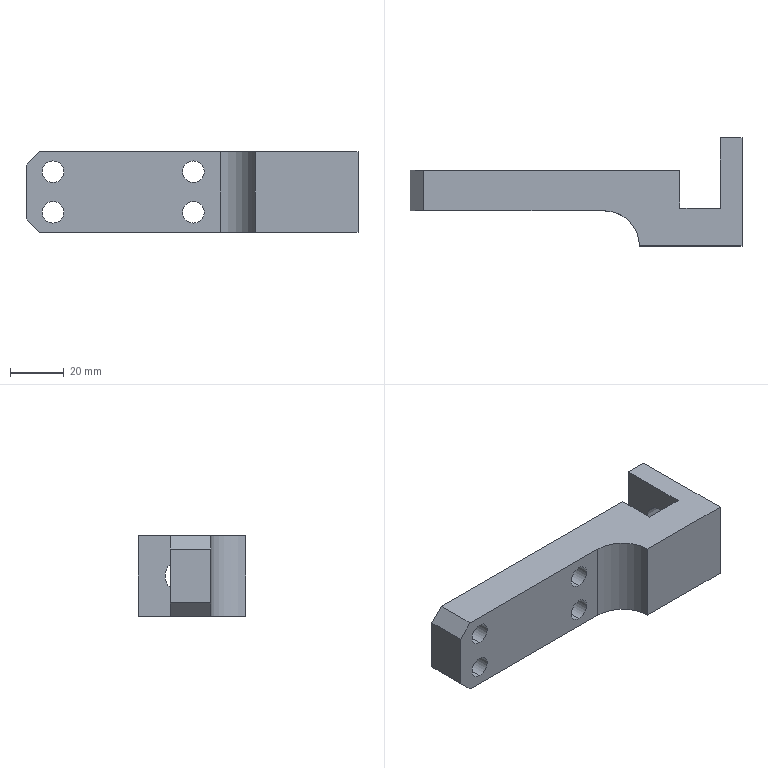Part | SolidWorks | features BaseBody 1 | 1 solid | 24 faces | box 123 x 40 x 30 mm | volume 63542 mm3 | plane 13 | cylinder 11 | commonest cylinder face diameters 8 x8 12 x2 26 x1
STEP:
#1=CARTESIAN_POINT('',(-340.,-80.,193.121));
#2=VERTEX_POINT('',#1);
#3=CARTESIAN_POINT('',(-340.,-80.,201.121));
#4=VERTEX_POINT('',#3);
#5=CARTESIAN_POINT('',(-340.,-80.,197.121));
#6=DIRECTION('',(0.,1.,0.));
#7=DIRECTION('',(0.,0.,-1.));
#8=AXIS2_PLACEMENT_3D('',#5,#6,#7);
#9=CIRCLE('',#8,4.);
#10=EDGE_CURVE('',#2,#4,#9,.T.);
#11=ORIENTED_EDGE('',*,*,#10,.T.);
#12=CARTESIAN_POINT('',(-340.,-95.,201.121));
#13=VERTEX_POINT('',#12);
#14=CARTESIAN_POINT('',(-340.,-95.,201.121));
#15=DIRECTION('',(0.,-1.,0.));
#16=VECTOR('',#15,1000.);
#17=LINE('',#14,#16);
#18=EDGE_CURVE('',#4,#13,#17,.T.);
#19=ORIENTED_EDGE('',*,*,#18,.T.);
#20=CARTESIAN_POINT('',(-340.,-95.,193.121));
#21=VERTEX_POINT('',#20);
#22=CARTESIAN_POINT('',(-340.,-95.,197.121));
#23=DIRECTION('',(0.,1.,0.));
#24=DIRECTION('',(0.,0.,-1.));
#25=AXIS2_PLACEMENT_3D('',#22,#23,#24);
#26=CIRCLE('',#25,4.);
#27=EDGE_CURVE('',#21,#13,#26,.T.);
#28=ORIENTED_EDGE('',*,*,#27,.F.);
#29=CARTESIAN_POINT('',(-340.,-95.,193.121));
#30=DIRECTION('',(0.,-1.,0.));
#31=VECTOR('',#30,1000.);
#32=LINE('',#29,#31);
#33=EDGE_CURVE('',#2,#21,#32,.T.);
#34=ORIENTED_EDGE('',*,*,#33,.F.);
#35=EDGE_LOOP('',(#11,#19,#28,#34));
#36=FACE_OUTER_BOUND('',#35,.T.);
#37=CARTESIAN_POINT('',(-340.,-95.,197.121));
#38=DIRECTION('',(0.,-1.,0.));
#39=DIRECTION('',(0.,0.,-1.));
#40=AXIS2_PLACEMENT_3D('',#37,#38,#39);
#41=CYLINDRICAL_SURFACE('',#40,4.);
#42=ADVANCED_FACE('',(#36),#41,.F.);
#43=CARTESIAN_POINT('',(-340.,-80.,178.121));
#44=VERTEX_POINT('',#43);
#45=CARTESIAN_POINT('',(-340.,-80.,186.121));
#46=VERTEX_POINT('',#45);
#47=CARTESIAN_POINT('',(-340.,-80.,182.121));
#48=DIRECTION('',(0.,1.,0.));
#49=DIRECTION('',(0.,0.,-1.));
#50=AXIS2_PLACEMENT_3D('',#47,#48,#49);
#51=CIRCLE('',#50,4.);
#52=EDGE_CURVE('',#44,#46,#51,.T.);
#53=ORIENTED_EDGE('',*,*,#52,.T.);
#54=CARTESIAN_POINT('',(-340.,-95.,186.121));
#55=VERTEX_POINT('',#54);
#56=CARTESIAN_POINT('',(-340.,-95.,186.121));
#57=DIRECTION('',(0.,-1.,0.));
#58=VECTOR('',#57,1000.);
#59=LINE('',#56,#58);
#60=EDGE_CURVE('',#46,#55,#59,.T.);
#61=ORIENTED_EDGE('',*,*,#60,.T.);
#62=CARTESIAN_POINT('',(-340.,-95.,178.121));
#63=VERTEX_POINT('',#62);
#64=CARTESIAN_POINT('',(-340.,-95.,182.121));
#65=DIRECTION('',(0.,1.,0.));
#66=DIRECTION('',(0.,0.,-1.));
#67=AXIS2_PLACEMENT_3D('',#64,#65,#66);
#68=CIRCLE('',#67,4.);
#69=EDGE_CURVE('',#63,#55,#68,.T.);
#70=ORIENTED_EDGE('',*,*,#69,.F.);
#71=CARTESIAN_POINT('',(-340.,-95.,178.121));
#72=DIRECTION('',(0.,-1.,0.));
#73=VECTOR('',#72,1000.);
#74=LINE('',#71,#73);
#75=EDGE_CURVE('',#44,#63,#74,.T.);
#76=ORIENTED_EDGE('',*,*,#75,.F.);
#77=EDGE_LOOP('',(#53,#61,#70,#76));
#78=FACE_OUTER_BOUND('',#77,.T.);
#79=CARTESIAN_POINT('',(-340.,-95.,182.121));
#80=DIRECTION('',(0.,-1.,0.));
#81=DIRECTION('',(0.,0.,-1.));
#82=AXIS2_PLACEMENT_3D('',#79,#80,#81);
#83=CYLINDRICAL_SURFACE('',#82,4.);
#84=ADVANCED_FACE('',(#78),#83,.F.);
#85=CARTESIAN_POINT('',(-288.,-80.,178.121));
#86=VERTEX_POINT('',#85);
#87=CARTESIAN_POINT('',(-288.,-80.,186.121));
#88=VERTEX_POINT('',#87);
#89=CARTESIAN_POINT('',(-288.,-80.,182.121));
#90=DIRECTION('',(0.,1.,0.));
#91=DIRECTION('',(0.,0.,-1.));
#92=AXIS2_PLACEMENT_3D('',#89,#90,#91);
#93=CIRCLE('',#92,4.);
#94=EDGE_CURVE('',#86,#88,#93,.T.);
#95=ORIENTED_EDGE('',*,*,#94,.T.);
#96=CARTESIAN_POINT('',(-288.,-95.,186.121));
#97=VERTEX_POINT('',#96);
#98=CARTESIAN_POINT('',(-288.,-95.,186.121));
#99=DIRECTION('',(0.,-1.,0.));
#100=VECTOR('',#99,1000.);
#101=LINE('',#98,#100);
#102=EDGE_CURVE('',#88,#97,#101,.T.);
#103=ORIENTED_EDGE('',*,*,#102,.T.);
#104=CARTESIAN_POINT('',(-288.,-95.,178.121));
#105=VERTEX_POINT('',#104);
#106=CARTESIAN_POINT('',(-288.,-95.,182.121));
#107=DIRECTION('',(0.,1.,0.));
#108=DIRECTION('',(0.,0.,-1.));
#109=AXIS2_PLACEMENT_3D('',#106,#107,#108);
#110=CIRCLE('',#109,4.);
#111=EDGE_CURVE('',#105,#97,#110,.T.);
#112=ORIENTED_EDGE('',*,*,#111,.F.);
#113=CARTESIAN_POINT('',(-288.,-95.,178.121));
#114=DIRECTION('',(0.,-1.,0.));
#115=VECTOR('',#114,1000.);
#116=LINE('',#113,#115);
#117=EDGE_CURVE('',#86,#105,#116,.T.);
#118=ORIENTED_EDGE('',*,*,#117,.F.);
#119=EDGE_LOOP('',(#95,#103,#112,#118));
#120=FACE_OUTER_BOUND('',#119,.T.);
#121=CARTESIAN_POINT('',(-288.,-95.,182.121));
#122=DIRECTION('',(0.,-1.,0.));
#123=DIRECTION('',(0.,0.,-1.));
#124=AXIS2_PLACEMENT_3D('',#121,#122,#123);
#125=CYLINDRICAL_SURFACE('',#124,4.);
#126=ADVANCED_FACE('',(#120),#125,.F.);
#127=CARTESIAN_POINT('',(-288.,-80.,193.121));
#128=VERTEX_POINT('',#127);
#129=CARTESIAN_POINT('',(-288.,-80.,201.121));
#130=VERTEX_POINT('',#129);
#131=CARTESIAN_POINT('',(-288.,-80.,197.121));
#132=DIRECTION('',(0.,1.,0.));
#133=DIRECTION('',(0.,0.,-1.));
#134=AXIS2_PLACEMENT_3D('',#131,#132,#133);
#135=CIRCLE('',#134,4.);
#136=EDGE_CURVE('',#128,#130,#135,.T.);
#137=ORIENTED_EDGE('',*,*,#136,.T.);
#138=CARTESIAN_POINT('',(-288.,-95.,201.121));
#139=VERTEX_POINT('',#138);
#140=CARTESIAN_POINT('',(-288.,-95.,201.121));
#141=DIRECTION('',(0.,-1.,0.));
#142=VECTOR('',#141,1000.);
#143=LINE('',#140,#142);
#144=EDGE_CURVE('',#130,#139,#143,.T.);
#145=ORIENTED_EDGE('',*,*,#144,.T.);
#146=CARTESIAN_POINT('',(-288.,-95.,193.121));
#147=VERTEX_POINT('',#146);
#148=CARTESIAN_POINT('',(-288.,-95.,197.121));
#149=DIRECTION('',(0.,1.,0.));
#150=DIRECTION('',(0.,0.,-1.));
#151=AXIS2_PLACEMENT_3D('',#148,#149,#150);
#152=CIRCLE('',#151,4.);
#153=EDGE_CURVE('',#147,#139,#152,.T.);
#154=ORIENTED_EDGE('',*,*,#153,.F.);
#155=CARTESIAN_POINT('',(-288.,-95.,193.121));
#156=DIRECTION('',(0.,-1.,0.));
#157=VECTOR('',#156,1000.);
#158=LINE('',#155,#157);
#159=EDGE_CURVE('',#128,#147,#158,.T.);
#160=ORIENTED_EDGE('',*,*,#159,.F.);
#161=EDGE_LOOP('',(#137,#145,#154,#160));
#162=FACE_OUTER_BOUND('',#161,.T.);
#163=CARTESIAN_POINT('',(-288.,-95.,197.121));
#164=DIRECTION('',(0.,-1.,0.));
#165=DIRECTION('',(0.,0.,-1.));
#166=AXIS2_PLACEMENT_3D('',#163,#164,#165);
#167=CYLINDRICAL_SURFACE('',#166,4.);
#168=ADVANCED_FACE('',(#162),#167,.F.);
#169=CARTESIAN_POINT('',(-235.,-84.,183.621));
#170=VERTEX_POINT('',#169);
#171=CARTESIAN_POINT('',(-235.,-84.,195.621));
#172=VERTEX_POINT('',#171);
#173=CARTESIAN_POINT('',(-235.,-84.,189.621));
#174=DIRECTION('',(-1.,0.,0.));
#175=DIRECTION('',(0.,0.,-1.));
#176=AXIS2_PLACEMENT_3D('',#173,#174,#175);
#177=CIRCLE('',#176,6.);
#178=EDGE_CURVE('',#170,#172,#177,.T.);
#179=ORIENTED_EDGE('',*,*,#178,.T.);
#180=CARTESIAN_POINT('',(-227.,-84.,195.621));
#181=VERTEX_POINT('',#180);
#182=CARTESIAN_POINT('',(-251.971,-84.,195.621));
#183=DIRECTION('',(1.,0.,0.));
#184=VECTOR('',#183,1000.);
#185=LINE('',#182,#184);
#186=EDGE_CURVE('',#172,#181,#185,.T.);
#187=ORIENTED_EDGE('',*,*,#186,.T.);
#188=CARTESIAN_POINT('',(-227.,-84.,183.621));
#189=VERTEX_POINT('',#188);
#190=CARTESIAN_POINT('',(-227.,-84.,189.621));
#191=DIRECTION('',(1.,0.,0.));
#192=DIRECTION('',(0.,0.,-1.));
#193=AXIS2_PLACEMENT_3D('',#190,#191,#192);
#194=CIRCLE('',#193,6.);
#195=EDGE_CURVE('',#181,#189,#194,.T.);
#196=ORIENTED_EDGE('',*,*,#195,.T.);
#197=CARTESIAN_POINT('',(-251.971,-84.,183.621));
#198=DIRECTION('',(1.,0.,0.));
#199=VECTOR('',#198,1000.);
#200=LINE('',#197,#199);
#201=EDGE_CURVE('',#170,#189,#200,.T.);
#202=ORIENTED_EDGE('',*,*,#201,.F.);
#203=EDGE_LOOP('',(#179,#187,#196,#202));
#204=FACE_OUTER_BOUND('',#203,.T.);
#205=CARTESIAN_POINT('',(-251.971,-84.,189.621));
#206=DIRECTION('',(1.,0.,0.));
#207=DIRECTION('',(0.,0.,-1.));
#208=AXIS2_PLACEMENT_3D('',#205,#206,#207);
#209=CYLINDRICAL_SURFACE('',#208,6.);
#210=ADVANCED_FACE('',(#204),#209,.F.);
#211=CARTESIAN_POINT('',(-345.,-80.,204.621));
#212=VERTEX_POINT('',#211);
#213=CARTESIAN_POINT('',(-350.,-80.,199.621));
#214=VERTEX_POINT('',#213);
#215=CARTESIAN_POINT('',(-345.,-80.,204.621));
#216=DIRECTION('',(-0.7071,0.,-0.7071));
#217=VECTOR('',#216,1000.);
#218=LINE('',#215,#217);
#219=EDGE_CURVE('',#212,#214,#218,.T.);
#220=ORIENTED_EDGE('',*,*,#219,.F.);
#221=CARTESIAN_POINT('',(-250.,-80.,204.621));
#222=VERTEX_POINT('',#221);
#223=CARTESIAN_POINT('',(-350.,-80.,204.621));
#224=DIRECTION('',(-1.,0.,0.));
#225=VECTOR('',#224,1000.);
#226=LINE('',#223,#225);
#227=EDGE_CURVE('',#222,#212,#226,.T.);
#228=ORIENTED_EDGE('',*,*,#227,.F.);
#229=CARTESIAN_POINT('',(-250.,-80.,174.621));
#230=VERTEX_POINT('',#229);
#231=CARTESIAN_POINT('',(-250.,-80.,204.621));
#232=DIRECTION('',(0.,0.,1.));
#233=VECTOR('',#232,1000.);
#234=LINE('',#231,#233);
#235=EDGE_CURVE('',#230,#222,#234,.T.);
#236=ORIENTED_EDGE('',*,*,#235,.F.);
#237=CARTESIAN_POINT('',(-345.,-80.,174.621));
#238=VERTEX_POINT('',#237);
#239=CARTESIAN_POINT('',(-350.,-80.,174.621));
#240=DIRECTION('',(1.,0.,0.));
#241=VECTOR('',#240,1000.);
#242=LINE('',#239,#241);
#243=EDGE_CURVE('',#238,#230,#242,.T.);
#244=ORIENTED_EDGE('',*,*,#243,.F.);
#245=CARTESIAN_POINT('',(-350.,-80.,179.621));
#246=VERTEX_POINT('',#245);
#247=CARTESIAN_POINT('',(-350.,-80.,179.621));
#248=DIRECTION('',(0.7071,0.,-0.7071));
#249=VECTOR('',#248,1000.);
#250=LINE('',#247,#249);
#251=EDGE_CURVE('',#246,#238,#250,.T.);
#252=ORIENTED_EDGE('',*,*,#251,.F.);
#253=CARTESIAN_POINT('',(-350.,-80.,204.621));
#254=DIRECTION('',(0.,0.,-1.));
#255=VECTOR('',#254,1000.);
#256=LINE('',#253,#255);
#257=EDGE_CURVE('',#214,#246,#256,.T.);
#258=ORIENTED_EDGE('',*,*,#257,.F.);
#259=EDGE_LOOP('',(#220,#228,#236,#244,#252,#258));
#260=FACE_OUTER_BOUND('',#259,.T.);
#261=ORIENTED_EDGE('',*,*,#10,.F.);
#262=CARTESIAN_POINT('',(-340.,-80.,197.121));
#263=DIRECTION('',(0.,1.,0.));
#264=DIRECTION('',(0.,0.,-1.));
#265=AXIS2_PLACEMENT_3D('',#262,#263,#264);
#266=CIRCLE('',#265,4.);
#267=EDGE_CURVE('',#4,#2,#266,.T.);
#268=ORIENTED_EDGE('',*,*,#267,.F.);
#269=EDGE_LOOP('',(#261,#268));
#270=FACE_BOUND('',#269,.T.);
#271=ORIENTED_EDGE('',*,*,#52,.F.);
#272=CARTESIAN_POINT('',(-340.,-80.,182.121));
#273=DIRECTION('',(0.,1.,0.));
#274=DIRECTION('',(0.,0.,-1.));
#275=AXIS2_PLACEMENT_3D('',#272,#273,#274);
#276=CIRCLE('',#275,4.);
#277=EDGE_CURVE('',#46,#44,#276,.T.);
#278=ORIENTED_EDGE('',*,*,#277,.F.);
#279=EDGE_LOOP('',(#271,#278));
#280=FACE_BOUND('',#279,.T.);
#281=ORIENTED_EDGE('',*,*,#94,.F.);
#282=CARTESIAN_POINT('',(-288.,-80.,182.121));
#283=DIRECTION('',(0.,1.,0.));
#284=DIRECTION('',(0.,0.,-1.));
#285=AXIS2_PLACEMENT_3D('',#282,#283,#284);
#286=CIRCLE('',#285,4.);
#287=EDGE_CURVE('',#88,#86,#286,.T.);
#288=ORIENTED_EDGE('',*,*,#287,.F.);
#289=EDGE_LOOP('',(#281,#288));
#290=FACE_BOUND('',#289,.T.);
#291=ORIENTED_EDGE('',*,*,#136,.F.);
#292=CARTESIAN_POINT('',(-288.,-80.,197.121));
#293=DIRECTION('',(0.,1.,0.));
#294=DIRECTION('',(0.,0.,-1.));
#295=AXIS2_PLACEMENT_3D('',#292,#293,#294);
#296=CIRCLE('',#295,4.);
#297=EDGE_CURVE('',#130,#128,#296,.T.);
#298=ORIENTED_EDGE('',*,*,#297,.F.);
#299=EDGE_LOOP('',(#291,#298));
#300=FACE_BOUND('',#299,.T.);
#301=CARTESIAN_POINT('',(-350.,-80.,204.621));
#302=DIRECTION('',(0.,-1.,0.));
#303=DIRECTION('',(0.,0.,-1.));
#304=AXIS2_PLACEMENT_3D('',#301,#302,#303);
#305=PLANE('',#304);
#306=ADVANCED_FACE('',(#260,#270,#280,#290,#300),#305,.F.);
#307=CARTESIAN_POINT('',(-350.,-95.,199.621));
#308=VERTEX_POINT('',#307);
#309=CARTESIAN_POINT('',(-350.,-80.,199.621));
#310=DIRECTION('',(0.,-1.,0.));
#311=VECTOR('',#310,1000.);
#312=LINE('',#309,#311);
#313=EDGE_CURVE('',#214,#308,#312,.T.);
#314=ORIENTED_EDGE('',*,*,#313,.F.);
#315=ORIENTED_EDGE('',*,*,#257,.T.);
#316=CARTESIAN_POINT('',(-350.,-95.,179.621));
#317=VERTEX_POINT('',#316);
#318=CARTESIAN_POINT('',(-350.,-80.,179.621));
#319=DIRECTION('',(0.,1.,0.));
#320=VECTOR('',#319,1000.);
#321=LINE('',#318,#320);
#322=EDGE_CURVE('',#317,#246,#321,.T.);
#323=ORIENTED_EDGE('',*,*,#322,.F.);
#324=CARTESIAN_POINT('',(-350.,-95.,204.621));
#325=DIRECTION('',(0.,0.,-1.));
#326=VECTOR('',#325,1000.);
#327=LINE('',#324,#326);
#328=EDGE_CURVE('',#308,#317,#327,.T.);
#329=ORIENTED_EDGE('',*,*,#328,.F.);
#330=EDGE_LOOP('',(#314,#315,#323,#329));
#331=FACE_OUTER_BOUND('',#330,.T.);
#332=CARTESIAN_POINT('',(-350.,-80.,204.621));
#333=DIRECTION('',(1.,0.,0.));
#334=DIRECTION('',(0.,0.,-1.));
#335=AXIS2_PLACEMENT_3D('',#332,#333,#334);
#336=PLANE('',#335);
#337=ADVANCED_FACE('',(#331),#336,.F.);
#338=CARTESIAN_POINT('',(-345.,-95.,204.621));
#339=VERTEX_POINT('',#338);
#340=CARTESIAN_POINT('',(-345.,-95.,204.621));
#341=DIRECTION('',(0.7071,0.,0.7071));
#342=VECTOR('',#341,1000.);
#343=LINE('',#340,#342);
#344=EDGE_CURVE('',#308,#339,#343,.T.);
#345=ORIENTED_EDGE('',*,*,#344,.T.);
#346=CARTESIAN_POINT('',(-345.,-82.6,204.621));
#347=DIRECTION('',(0.,1.,0.));
#348=VECTOR('',#347,1000.);
#349=LINE('',#346,#348);
#350=EDGE_CURVE('',#339,#212,#349,.T.);
#351=ORIENTED_EDGE('',*,*,#350,.T.);
#352=ORIENTED_EDGE('',*,*,#219,.T.);
#353=ORIENTED_EDGE('',*,*,#313,.T.);
#354=EDGE_LOOP('',(#345,#351,#352,#353));
#355=FACE_OUTER_BOUND('',#354,.T.);
#356=CARTESIAN_POINT('',(-345.,-82.6,204.621));
#357=DIRECTION('',(-0.7071,0.,0.7071));
#358=DIRECTION('',(0.7071,0.,0.7071));
#359=AXIS2_PLACEMENT_3D('',#356,#357,#358);
#360=PLANE('',#359);
#361=ADVANCED_FACE('',(#355),#360,.T.);
#362=CARTESIAN_POINT('',(-235.,-94.,204.621));
#363=VERTEX_POINT('',#362);
#364=CARTESIAN_POINT('',(-250.,-94.,204.621));
#365=VERTEX_POINT('',#364);
#366=CARTESIAN_POINT('',(-251.867,-94.,204.621));
#367=DIRECTION('',(-1.,0.,0.));
#368=VECTOR('',#367,1000.);
#369=LINE('',#366,#368);
#370=EDGE_CURVE('',#363,#365,#369,.T.);
#371=ORIENTED_EDGE('',*,*,#370,.T.);
#372=CARTESIAN_POINT('',(-250.,-82.6,204.621));
#373=DIRECTION('',(0.,1.,0.));
#374=VECTOR('',#373,1000.);
#375=LINE('',#372,#374);
#376=EDGE_CURVE('',#365,#222,#375,.T.);
#377=ORIENTED_EDGE('',*,*,#376,.T.);
#378=ORIENTED_EDGE('',*,*,#227,.T.);
#379=ORIENTED_EDGE('',*,*,#350,.F.);
#380=CARTESIAN_POINT('',(-278.,-95.,204.621));
#381=VERTEX_POINT('',#380);
#382=CARTESIAN_POINT('',(-251.867,-95.,204.621));
#383=DIRECTION('',(1.,0.,0.));
#384=VECTOR('',#383,1000.);
#385=LINE('',#382,#384);
#386=EDGE_CURVE('',#339,#381,#385,.T.);
#387=ORIENTED_EDGE('',*,*,#386,.T.);
#388=CARTESIAN_POINT('',(-265.,-108.,204.621));
#389=VERTEX_POINT('',#388);
#390=CARTESIAN_POINT('',(-278.,-108.,204.621));
#391=DIRECTION('',(0.,0.,-1.));
#392=DIRECTION('',(1.,0.,0.));
#393=AXIS2_PLACEMENT_3D('',#390,#391,#392);
#394=CIRCLE('',#393,13.);
#395=EDGE_CURVE('',#381,#389,#394,.T.);
#396=ORIENTED_EDGE('',*,*,#395,.T.);
#397=CARTESIAN_POINT('',(-227.,-108.,204.621));
#398=VERTEX_POINT('',#397);
#399=CARTESIAN_POINT('',(-251.867,-108.,204.621));
#400=DIRECTION('',(1.,0.,0.));
#401=VECTOR('',#400,1000.);
#402=LINE('',#399,#401);
#403=EDGE_CURVE('',#389,#398,#402,.T.);
#404=ORIENTED_EDGE('',*,*,#403,.T.);
#405=CARTESIAN_POINT('',(-227.,-68.,204.621));
#406=VERTEX_POINT('',#405);
#407=CARTESIAN_POINT('',(-227.,-82.6,204.621));
#408=DIRECTION('',(0.,1.,0.));
#409=VECTOR('',#408,1000.);
#410=LINE('',#407,#409);
#411=EDGE_CURVE('',#398,#406,#410,.T.);
#412=ORIENTED_EDGE('',*,*,#411,.T.);
#413=CARTESIAN_POINT('',(-235.,-68.,204.621));
#414=VERTEX_POINT('',#413);
#415=CARTESIAN_POINT('',(-251.867,-68.,204.621));
#416=DIRECTION('',(-1.,0.,0.));
#417=VECTOR('',#416,1000.);
#418=LINE('',#415,#417);
#419=EDGE_CURVE('',#406,#414,#418,.T.);
#420=ORIENTED_EDGE('',*,*,#419,.T.);
#421=CARTESIAN_POINT('',(-235.,-82.6,204.621));
#422=DIRECTION('',(0.,-1.,0.));
#423=VECTOR('',#422,1000.);
#424=LINE('',#421,#423);
#425=EDGE_CURVE('',#414,#363,#424,.T.);
#426=ORIENTED_EDGE('',*,*,#425,.T.);
#427=EDGE_LOOP('',(#371,#377,#378,#379,#387,#396,#404,#412,#420,#426));
#428=FACE_OUTER_BOUND('',#427,.T.);
#429=CARTESIAN_POINT('',(-251.867,-82.6,204.621));
#430=DIRECTION('',(0.,0.,1.));
#431=DIRECTION('',(1.,0.,0.));
#432=AXIS2_PLACEMENT_3D('',#429,#430,#431);
#433=PLANE('',#432);
#434=ADVANCED_FACE('',(#428),#433,.T.);
#435=ORIENTED_EDGE('',*,*,#235,.T.);
#436=ORIENTED_EDGE('',*,*,#376,.F.);
#437=CARTESIAN_POINT('',(-250.,-94.,174.621));
#438=VERTEX_POINT('',#437);
#439=CARTESIAN_POINT('',(-250.,-94.,204.621));
#440=DIRECTION('',(0.,0.,1.));
#441=VECTOR('',#440,1000.);
#442=LINE('',#439,#441);
#443=EDGE_CURVE('',#438,#365,#442,.T.);
#444=ORIENTED_EDGE('',*,*,#443,.F.);
#445=CARTESIAN_POINT('',(-250.,-80.,174.621));
#446=DIRECTION('',(0.,-1.,0.));
#447=VECTOR('',#446,1000.);
#448=LINE('',#445,#447);
#449=EDGE_CURVE('',#230,#438,#448,.T.);
#450=ORIENTED_EDGE('',*,*,#449,.F.);
#451=EDGE_LOOP('',(#435,#436,#444,#450));
#452=FACE_OUTER_BOUND('',#451,.T.);
#453=CARTESIAN_POINT('',(-250.,-80.,204.621));
#454=DIRECTION('',(-1.,0.,0.));
#455=DIRECTION('',(0.,0.,1.));
#456=AXIS2_PLACEMENT_3D('',#453,#454,#455);
#457=PLANE('',#456);
#458=ADVANCED_FACE('',(#452),#457,.F.);
#459=CARTESIAN_POINT('',(-345.,-95.,174.621));
#460=VERTEX_POINT('',#459);
#461=CARTESIAN_POINT('',(-345.,-82.6,174.621));
#462=DIRECTION('',(0.,-1.,0.));
#463=VECTOR('',#462,1000.);
#464=LINE('',#461,#463);
#465=EDGE_CURVE('',#238,#460,#464,.T.);
#466=ORIENTED_EDGE('',*,*,#465,.F.);
#467=ORIENTED_EDGE('',*,*,#243,.T.);
#468=ORIENTED_EDGE('',*,*,#449,.T.);
#469=CARTESIAN_POINT('',(-235.,-94.,174.621));
#470=VERTEX_POINT('',#469);
#471=CARTESIAN_POINT('',(-251.867,-94.,174.621));
#472=DIRECTION('',(-1.,0.,0.));
#473=VECTOR('',#472,1000.);
#474=LINE('',#471,#473);
#475=EDGE_CURVE('',#470,#438,#474,.T.);
#476=ORIENTED_EDGE('',*,*,#475,.F.);
#477=CARTESIAN_POINT('',(-235.,-68.,174.621));
#478=VERTEX_POINT('',#477);
#479=CARTESIAN_POINT('',(-235.,-82.6,174.621));
#480=DIRECTION('',(0.,-1.,0.));
#481=VECTOR('',#480,1000.);
#482=LINE('',#479,#481);
#483=EDGE_CURVE('',#478,#470,#482,.T.);
#484=ORIENTED_EDGE('',*,*,#483,.F.);
#485=CARTESIAN_POINT('',(-227.,-68.,174.621));
#486=VERTEX_POINT('',#485);
#487=CARTESIAN_POINT('',(-251.867,-68.,174.621));
#488=DIRECTION('',(-1.,0.,0.));
#489=VECTOR('',#488,1000.);
#490=LINE('',#487,#489);
#491=EDGE_CURVE('',#486,#478,#490,.T.);
#492=ORIENTED_EDGE('',*,*,#491,.F.);
#493=CARTESIAN_POINT('',(-227.,-108.,174.621));
#494=VERTEX_POINT('',#493);
#495=CARTESIAN_POINT('',(-227.,-82.6,174.621));
#496=DIRECTION('',(0.,1.,0.));
#497=VECTOR('',#496,1000.);
#498=LINE('',#495,#497);
#499=EDGE_CURVE('',#494,#486,#498,.T.);
#500=ORIENTED_EDGE('',*,*,#499,.F.);
#501=CARTESIAN_POINT('',(-265.,-108.,174.621));
#502=VERTEX_POINT('',#501);
#503=CARTESIAN_POINT('',(-251.867,-108.,174.621));
#504=DIRECTION('',(1.,0.,0.));
#505=VECTOR('',#504,1000.);
#506=LINE('',#503,#505);
#507=EDGE_CURVE('',#502,#494,#506,.T.);
#508=ORIENTED_EDGE('',*,*,#507,.F.);
#509=CARTESIAN_POINT('',(-278.,-95.,174.621));
#510=VERTEX_POINT('',#509);
#511=CARTESIAN_POINT('',(-278.,-108.,174.621));
#512=DIRECTION('',(0.,0.,-1.));
#513=DIRECTION('',(1.,0.,0.));
#514=AXIS2_PLACEMENT_3D('',#511,#512,#513);
#515=CIRCLE('',#514,13.);
#516=EDGE_CURVE('',#510,#502,#515,.T.);
#517=ORIENTED_EDGE('',*,*,#516,.F.);
#518=CARTESIAN_POINT('',(-251.867,-95.,174.621));
#519=DIRECTION('',(1.,0.,0.));
#520=VECTOR('',#519,1000.);
#521=LINE('',#518,#520);
#522=EDGE_CURVE('',#460,#510,#521,.T.);
#523=ORIENTED_EDGE('',*,*,#522,.F.);
#524=EDGE_LOOP('',(#466,#467,#468,#476,#484,#492,#500,#508,#517,#523));
#525=FACE_OUTER_BOUND('',#524,.T.);
#526=CARTESIAN_POINT('',(-251.867,-82.6,174.621));
#527=DIRECTION('',(0.,0.,1.));
#528=DIRECTION('',(1.,0.,0.));
#529=AXIS2_PLACEMENT_3D('',#526,#527,#528);
#530=PLANE('',#529);
#531=ADVANCED_FACE('',(#525),#530,.F.);
#532=ORIENTED_EDGE('',*,*,#465,.T.);
#533=CARTESIAN_POINT('',(-350.,-95.,179.621));
#534=DIRECTION('',(0.7071,0.,-0.7071));
#535=VECTOR('',#534,1000.);
#536=LINE('',#533,#535);
#537=EDGE_CURVE('',#317,#460,#536,.T.);
#538=ORIENTED_EDGE('',*,*,#537,.F.);
#539=ORIENTED_EDGE('',*,*,#322,.T.);
#540=ORIENTED_EDGE('',*,*,#251,.T.);
#541=EDGE_LOOP('',(#532,#538,#539,#540));
#542=FACE_OUTER_BOUND('',#541,.T.);
#543=CARTESIAN_POINT('',(-350.,-80.,179.621));
#544=DIRECTION('',(0.7071,0.,0.7071));
#545=DIRECTION('',(0.7071,0.,-0.7071));
#546=AXIS2_PLACEMENT_3D('',#543,#544,#545);
#547=PLANE('',#546);
#548=ADVANCED_FACE('',(#542),#547,.F.);
#549=ORIENTED_EDGE('',*,*,#18,.F.);
#550=ORIENTED_EDGE('',*,*,#267,.T.);
#551=ORIENTED_EDGE('',*,*,#33,.T.);
#552=CARTESIAN_POINT('',(-340.,-95.,197.121));
#553=DIRECTION('',(0.,1.,0.));
#554=DIRECTION('',(0.,0.,-1.));
#555=AXIS2_PLACEMENT_3D('',#552,#553,#554);
#556=CIRCLE('',#555,4.);
#557=EDGE_CURVE('',#13,#21,#556,.T.);
#558=ORIENTED_EDGE('',*,*,#557,.F.);
#559=EDGE_LOOP('',(#549,#550,#551,#558));
#560=FACE_OUTER_BOUND('',#559,.T.);
#561=CARTESIAN_POINT('',(-340.,-95.,197.121));
#562=DIRECTION('',(0.,-1.,0.));
#563=DIRECTION('',(0.,0.,-1.));
#564=AXIS2_PLACEMENT_3D('',#561,#562,#563);
#565=CYLINDRICAL_SURFACE('',#564,4.);
#566=ADVANCED_FACE('',(#560),#565,.F.);
#567=ORIENTED_EDGE('',*,*,#60,.F.);
#568=ORIENTED_EDGE('',*,*,#277,.T.);
#569=ORIENTED_EDGE('',*,*,#75,.T.);
#570=CARTESIAN_POINT('',(-340.,-95.,182.121));
#571=DIRECTION('',(0.,1.,0.));
#572=DIRECTION('',(0.,0.,-1.));
#573=AXIS2_PLACEMENT_3D('',#570,#571,#572);
#574=CIRCLE('',#573,4.);
#575=EDGE_CURVE('',#55,#63,#574,.T.);
#576=ORIENTED_EDGE('',*,*,#575,.F.);
#577=EDGE_LOOP('',(#567,#568,#569,#576));
#578=FACE_OUTER_BOUND('',#577,.T.);
#579=CARTESIAN_POINT('',(-340.,-95.,182.121));
#580=DIRECTION('',(0.,-1.,0.));
#581=DIRECTION('',(0.,0.,-1.));
#582=AXIS2_PLACEMENT_3D('',#579,#580,#581);
#583=CYLINDRICAL_SURFACE('',#582,4.);
#584=ADVANCED_FACE('',(#578),#583,.F.);
#585=ORIENTED_EDGE('',*,*,#102,.F.);
#586=ORIENTED_EDGE('',*,*,#287,.T.);
#587=ORIENTED_EDGE('',*,*,#117,.T.);
#588=CARTESIAN_POINT('',(-288.,-95.,182.121));
#589=DIRECTION('',(0.,1.,0.));
#590=DIRECTION('',(0.,0.,-1.));
#591=AXIS2_PLACEMENT_3D('',#588,#589,#590);
#592=CIRCLE('',#591,4.);
#593=EDGE_CURVE('',#97,#105,#592,.T.);
#594=ORIENTED_EDGE('',*,*,#593,.F.);
#595=EDGE_LOOP('',(#585,#586,#587,#594));
#596=FACE_OUTER_BOUND('',#595,.T.);
#597=CARTESIAN_POINT('',(-288.,-95.,182.121));
#598=DIRECTION('',(0.,-1.,0.));
#599=DIRECTION('',(0.,0.,-1.));
#600=AXIS2_PLACEMENT_3D('',#597,#598,#599);
#601=CYLINDRICAL_SURFACE('',#600,4.);
#602=ADVANCED_FACE('',(#596),#601,.F.);
#603=ORIENTED_EDGE('',*,*,#144,.F.);
#604=ORIENTED_EDGE('',*,*,#297,.T.);
#605=ORIENTED_EDGE('',*,*,#159,.T.);
#606=CARTESIAN_POINT('',(-288.,-95.,197.121));
#607=DIRECTION('',(0.,1.,0.));
#608=DIRECTION('',(0.,0.,-1.));
#609=AXIS2_PLACEMENT_3D('',#606,#607,#608);
#610=CIRCLE('',#609,4.);
#611=EDGE_CURVE('',#139,#147,#610,.T.);
#612=ORIENTED_EDGE('',*,*,#611,.F.);
#613=EDGE_LOOP('',(#603,#604,#605,#612));
#614=FACE_OUTER_BOUND('',#613,.T.);
#615=CARTESIAN_POINT('',(-288.,-95.,197.121));
#616=DIRECTION('',(0.,-1.,0.));
#617=DIRECTION('',(0.,0.,-1.));
#618=AXIS2_PLACEMENT_3D('',#615,#616,#617);
#619=CYLINDRICAL_SURFACE('',#618,4.);
#620=ADVANCED_FACE('',(#614),#619,.F.);
#621=ORIENTED_EDGE('',*,*,#344,.F.);
#622=ORIENTED_EDGE('',*,*,#328,.T.);
#623=ORIENTED_EDGE('',*,*,#537,.T.);
#624=ORIENTED_EDGE('',*,*,#522,.T.);
#625=CARTESIAN_POINT('',(-278.,-95.,204.621));
#626=DIRECTION('',(0.,0.,-1.));
#627=VECTOR('',#626,1000.);
#628=LINE('',#625,#627);
#629=EDGE_CURVE('',#381,#510,#628,.T.);
#630=ORIENTED_EDGE('',*,*,#629,.F.);
#631=ORIENTED_EDGE('',*,*,#386,.F.);
#632=EDGE_LOOP('',(#621,#622,#623,#624,#630,#631));
#633=FACE_OUTER_BOUND('',#632,.T.);
#634=ORIENTED_EDGE('',*,*,#27,.T.);
#635=ORIENTED_EDGE('',*,*,#557,.T.);
#636=EDGE_LOOP('',(#634,#635));
#637=FACE_BOUND('',#636,.T.);
#638=ORIENTED_EDGE('',*,*,#69,.T.);
#639=ORIENTED_EDGE('',*,*,#575,.T.);
#640=EDGE_LOOP('',(#638,#639));
#641=FACE_BOUND('',#640,.T.);
#642=ORIENTED_EDGE('',*,*,#111,.T.);
#643=ORIENTED_EDGE('',*,*,#593,.T.);
#644=EDGE_LOOP('',(#642,#643));
#645=FACE_BOUND('',#644,.T.);
#646=ORIENTED_EDGE('',*,*,#153,.T.);
#647=ORIENTED_EDGE('',*,*,#611,.T.);
#648=EDGE_LOOP('',(#646,#647));
#649=FACE_BOUND('',#648,.T.);
#650=CARTESIAN_POINT('',(-350.,-95.,204.621));
#651=DIRECTION('',(0.,1.,0.));
#652=DIRECTION('',(0.,0.,1.));
#653=AXIS2_PLACEMENT_3D('',#650,#651,#652);
#654=PLANE('',#653);
#655=ADVANCED_FACE('',(#633,#637,#641,#645,#649),#654,.F.);
#656=ORIENTED_EDGE('',*,*,#443,.T.);
#657=ORIENTED_EDGE('',*,*,#370,.F.);
#658=CARTESIAN_POINT('',(-235.,-94.,204.621));
#659=DIRECTION('',(0.,0.,1.));
#660=VECTOR('',#659,1000.);
#661=LINE('',#658,#660);
#662=EDGE_CURVE('',#470,#363,#661,.T.);
#663=ORIENTED_EDGE('',*,*,#662,.F.);
#664=ORIENTED_EDGE('',*,*,#475,.T.);
#665=EDGE_LOOP('',(#656,#657,#663,#664));
#666=FACE_OUTER_BOUND('',#665,.T.);
#667=CARTESIAN_POINT('',(-250.,-94.,204.621));
#668=DIRECTION('',(0.,-1.,0.));
#669=DIRECTION('',(0.,0.,-1.));
#670=AXIS2_PLACEMENT_3D('',#667,#668,#669);
#671=PLANE('',#670);
#672=ADVANCED_FACE('',(#666),#671,.F.);
#673=ORIENTED_EDGE('',*,*,#662,.T.);
#674=ORIENTED_EDGE('',*,*,#425,.F.);
#675=CARTESIAN_POINT('',(-235.,-68.,204.621));
#676=DIRECTION('',(0.,0.,1.));
#677=VECTOR('',#676,1000.);
#678=LINE('',#675,#677);
#679=EDGE_CURVE('',#478,#414,#678,.T.);
#680=ORIENTED_EDGE('',*,*,#679,.F.);
#681=ORIENTED_EDGE('',*,*,#483,.T.);
#682=EDGE_LOOP('',(#673,#674,#680,#681));
#683=FACE_OUTER_BOUND('',#682,.T.);
#684=ORIENTED_EDGE('',*,*,#178,.F.);
#685=CARTESIAN_POINT('',(-235.,-84.,189.621));
#686=DIRECTION('',(-1.,0.,0.));
#687=DIRECTION('',(0.,0.,-1.));
#688=AXIS2_PLACEMENT_3D('',#685,#686,#687);
#689=CIRCLE('',#688,6.);
#690=EDGE_CURVE('',#172,#170,#689,.T.);
#691=ORIENTED_EDGE('',*,*,#690,.F.);
#692=EDGE_LOOP('',(#684,#691));
#693=FACE_BOUND('',#692,.T.);
#694=CARTESIAN_POINT('',(-235.,-94.,204.621));
#695=DIRECTION('',(1.,0.,0.));
#696=DIRECTION('',(0.,0.,-1.));
#697=AXIS2_PLACEMENT_3D('',#694,#695,#696);
#698=PLANE('',#697);
#699=ADVANCED_FACE('',(#683,#693),#698,.F.);
#700=ORIENTED_EDGE('',*,*,#679,.T.);
#701=ORIENTED_EDGE('',*,*,#419,.F.);
#702=CARTESIAN_POINT('',(-227.,-68.,204.621));
#703=DIRECTION('',(0.,0.,1.));
#704=VECTOR('',#703,1000.);
#705=LINE('',#702,#704);
#706=EDGE_CURVE('',#486,#406,#705,.T.);
#707=ORIENTED_EDGE('',*,*,#706,.F.);
#708=ORIENTED_EDGE('',*,*,#491,.T.);
#709=EDGE_LOOP('',(#700,#701,#707,#708));
#710=FACE_OUTER_BOUND('',#709,.T.);
#711=CARTESIAN_POINT('',(-227.,-68.,204.621));
#712=DIRECTION('',(0.,-1.,0.));
#713=DIRECTION('',(0.,0.,-1.));
#714=AXIS2_PLACEMENT_3D('',#711,#712,#713);
#715=PLANE('',#714);
#716=ADVANCED_FACE('',(#710),#715,.F.);
#717=ORIENTED_EDGE('',*,*,#706,.T.);
#718=ORIENTED_EDGE('',*,*,#411,.F.);
#719=CARTESIAN_POINT('',(-227.,-108.,204.621));
#720=DIRECTION('',(0.,0.,1.));
#721=VECTOR('',#720,1000.);
#722=LINE('',#719,#721);
#723=EDGE_CURVE('',#494,#398,#722,.T.);
#724=ORIENTED_EDGE('',*,*,#723,.F.);
#725=ORIENTED_EDGE('',*,*,#499,.T.);
#726=EDGE_LOOP('',(#717,#718,#724,#725));
#727=FACE_OUTER_BOUND('',#726,.T.);
#728=CARTESIAN_POINT('',(-227.,-84.,189.621));
#729=DIRECTION('',(1.,0.,0.));
#730=DIRECTION('',(0.,0.,-1.));
#731=AXIS2_PLACEMENT_3D('',#728,#729,#730);
#732=CIRCLE('',#731,6.);
#733=EDGE_CURVE('',#189,#181,#732,.T.);
#734=ORIENTED_EDGE('',*,*,#733,.F.);
#735=ORIENTED_EDGE('',*,*,#195,.F.);
#736=EDGE_LOOP('',(#734,#735));
#737=FACE_BOUND('',#736,.T.);
#738=CARTESIAN_POINT('',(-227.,-93.,204.621));
#739=DIRECTION('',(-1.,0.,0.));
#740=DIRECTION('',(0.,0.,1.));
#741=AXIS2_PLACEMENT_3D('',#738,#739,#740);
#742=PLANE('',#741);
#743=ADVANCED_FACE('',(#727,#737),#742,.F.);
#744=ORIENTED_EDGE('',*,*,#723,.T.);
#745=ORIENTED_EDGE('',*,*,#403,.F.);
#746=CARTESIAN_POINT('',(-265.,-108.,204.621));
#747=DIRECTION('',(0.,0.,1.));
#748=VECTOR('',#747,1000.);
#749=LINE('',#746,#748);
#750=EDGE_CURVE('',#502,#389,#749,.T.);
#751=ORIENTED_EDGE('',*,*,#750,.F.);
#752=ORIENTED_EDGE('',*,*,#507,.T.);
#753=EDGE_LOOP('',(#744,#745,#751,#752));
#754=FACE_OUTER_BOUND('',#753,.T.);
#755=CARTESIAN_POINT('',(-265.,-108.,204.621));
#756=DIRECTION('',(0.,1.,0.));
#757=DIRECTION('',(0.,0.,1.));
#758=AXIS2_PLACEMENT_3D('',#755,#756,#757);
#759=PLANE('',#758);
#760=ADVANCED_FACE('',(#754),#759,.F.);
#761=ORIENTED_EDGE('',*,*,#629,.T.);
#762=ORIENTED_EDGE('',*,*,#516,.T.);
#763=ORIENTED_EDGE('',*,*,#750,.T.);
#764=ORIENTED_EDGE('',*,*,#395,.F.);
#765=EDGE_LOOP('',(#761,#762,#763,#764));
#766=FACE_OUTER_BOUND('',#765,.T.);
#767=CARTESIAN_POINT('',(-278.,-108.,204.621));
#768=DIRECTION('',(0.,0.,1.));
#769=DIRECTION('',(1.,0.,0.));
#770=AXIS2_PLACEMENT_3D('',#767,#768,#769);
#771=CYLINDRICAL_SURFACE('',#770,13.);
#772=ADVANCED_FACE('',(#766),#771,.F.);
#773=ORIENTED_EDGE('',*,*,#186,.F.);
#774=ORIENTED_EDGE('',*,*,#690,.T.);
#775=ORIENTED_EDGE('',*,*,#201,.T.);
#776=ORIENTED_EDGE('',*,*,#733,.T.);
#777=EDGE_LOOP('',(#773,#774,#775,#776));
#778=FACE_OUTER_BOUND('',#777,.T.);
#779=CARTESIAN_POINT('',(-251.971,-84.,189.621));
#780=DIRECTION('',(1.,0.,0.));
#781=DIRECTION('',(0.,0.,-1.));
#782=AXIS2_PLACEMENT_3D('',#779,#780,#781);
#783=CYLINDRICAL_SURFACE('',#782,6.);
#784=ADVANCED_FACE('',(#778),#783,.F.);
#785=CLOSED_SHELL('',(#42,#84,#126,#168,#210,#306,#337,#361,#434,#458,#531,#548,#566,#584,#602,#620,#655,#672,#699,#716,#743,#760,#772,#784));
#786=MANIFOLD_SOLID_BREP('',#785);
#787=CARTESIAN_POINT('',(0.,0.,0.));
#788=DIRECTION('',(0.,0.,1.));
#789=DIRECTION('',(1.,0.,0.));
#790=AXIS2_PLACEMENT_3D('',#787,#788,#789);
#791=(LENGTH_UNIT()NAMED_UNIT(*)SI_UNIT(.MILLI.,.METRE.));
#792=UNCERTAINTY_MEASURE_WITH_UNIT(LENGTH_MEASURE(0.00001),#791,'','');
#793=(NAMED_UNIT(*)PLANE_ANGLE_UNIT()SI_UNIT($,.RADIAN.));
#794=(NAMED_UNIT(*)SI_UNIT($,.STERADIAN.)SOLID_ANGLE_UNIT());
#795=(GEOMETRIC_REPRESENTATION_CONTEXT(3)GLOBAL_UNCERTAINTY_ASSIGNED_CONTEXT((#792))GLOBAL_UNIT_ASSIGNED_CONTEXT((#791,#793,#794))REPRESENTATION_CONTEXT('',''));
#796=ADVANCED_BREP_SHAPE_REPRESENTATION('',(#786,#790),#795);